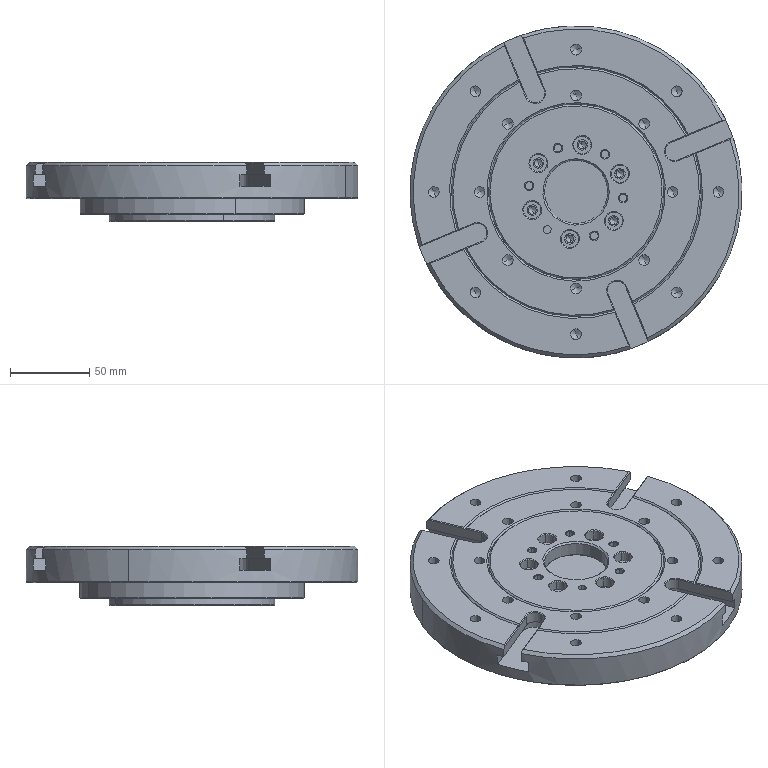NC program | Mastercam | posted with a generic post
Lines 3021 to 3620 of 4738:
(8 FEMF |TOOL - 9|DIA. OFF. - 9|LEN. - 9|TOOL DIA. - 8.)
N6098 T9 M6
N6100 G0 G54 G90 X17.184 Y2.469 C0. B0. S3500 M3
N6102 G43 H9 Z64.45
N6104 Z15.45
N6106 G1 Z14.45 F2000.
N6108 G41 D9 X14.616 Y-.598 F600.
N6110 G3 X14.594 Y-.645 I.077 J-.065
N6112 G1 X14.035 Y-3.838
N6114 X13.662 Y-4.467
N6116 G2 X.255 Y-12.103 I-13.407 J7.951
N6118 X-.045 Y-12.1 J15.587
N6120 X-12.1 Y0. I.045 J12.1
N6122 X-8.614 Y8.498 I12.1
N6124 G3 X-8.588 Y8.543 I-.071 J.07
N6126 G1 G40 X-7.579 Y12.413
N6128 G0 Z64.45
N6130 X17.184 Y2.469
N6132 Z15.45
N6134 G1 Z14.45 F2000.
N6136 G41 D9 X14.616 Y-.598 F600.
N6138 G3 X14.594 Y-.645 I.077 J-.065
N6140 G1 X14.035 Y-3.838
N6142 X13.662 Y-4.467
N6144 G2 X.255 Y-12.103 I-13.407 J7.951
N6146 X-.045 Y-12.1 J15.587
N6148 X-12.1 Y0. I.045 J12.1
N6150 X-8.614 Y8.498 I12.1
N6152 G3 X-8.588 Y8.543 I-.071 J.07
N6154 G1 G40 X-7.579 Y12.413
N6156 G0 Z64.45
N6158 C8.2 B-90.
N6160 X9.88 Y12.106
N6162 Z52.35
N6164 Z3.35
N6166 G1 Z2.35 F2000.
N6168 G41 D9 X9.521 Y8.122 F600.
N6170 G3 X9.5 Y7.657 I5.159 J-.465
N6172 X10.533 Y4.554 I5.18
N6174 G2 X12.001 Y.143 I-5.895 J-4.411
N6176 X10.828 Y-3.842 I-7.363
N6178 G3 X9.494 Y-8.378 I7.046 J-4.536
N6180 X9.5 Y-8.689 I8.38
N6182 G1 G40 X9.649 Y-12.687
N6184 G0 Z52.35
N6186 X9.88 Y12.106
N6188 Z3.35
N6190 G1 Z2.35 F2000.
N6192 G41 D9 X9.521 Y8.122 F600.
N6194 G3 X9.5 Y7.657 I5.159 J-.465
N6196 X10.533 Y4.554 I5.18
N6198 G2 X12.001 Y.143 I-5.895 J-4.411
N6200 X10.828 Y-3.842 I-7.363
N6202 G3 X9.494 Y-8.378 I7.046 J-4.536
N6204 X9.5 Y-8.689 I8.38
N6206 G1 G40 X9.649 Y-12.687
N6208 G0 Z52.35
N6210 X8.084 Y14.292
N6212 Z51.6
N6214 Z2.6
N6216 G1 Z-8.4 F2000.
N6218 G41 D9 X9.387 Y10.51 F600.
N6220 G3 X11.312 Y9.137 I1.925 J.663
N6222 X12.291 Y9.388 J2.036
N6224 G1 X18.686 Y13.541
N6226 G2 X21. Y14.226 I2.314 J-3.565
N6228 X25.25 Y9.976 J-4.25
N6230 X25.248 Y9.827 I-4.25
N6232 G1 Y9.82
N6234 G3 X25.44 Y9.62 I.199
N6236 G1 G40 X29.438 Y9.48
N6238 G0 Z41.6
N6240 X8.084 Y14.292
N6242 Z2.6
N6244 G1 Z-8.4 F2000.
N6246 G41 D9 X9.387 Y10.51 F600.
N6248 G3 X11.312 Y9.137 I1.925 J.663
N6250 X12.291 Y9.388 J2.036
N6252 G1 X18.686 Y13.541
N6254 G2 X21. Y14.226 I2.314 J-3.565
N6256 X25.25 Y9.976 J-4.25
N6258 X25.248 Y9.827 I-4.25
N6260 G1 Y9.82
N6262 G3 X25.44 Y9.62 I.199
N6264 G1 G40 X29.438 Y9.48
N6266 G0 Z51.6
N6268 Z57.06
N6270 X7.26 Y7.762
N6272 C0.
N6274 Z8.06
N6276 G1 Z7.06 F2000.
N6278 G41 D9 Y3.762 F600.
N6280 Y-3.762
N6282 G40 Y-7.762
N6284 G0 Z57.06
N6286 S3000 M3
N6288 C-.095 B-87.702
N6290 X25.467 Y13.177
N6292 Z42.615
N6294 Z-6.385
N6296 G1 Z-7.385 F2000.
N6298 G41 D9 X25.384 Y11.178 F400.
N6300 X24.716 Y-4.985
N6302 G40 X24.634 Y-6.983
N6304 G0 Z42.615
N6306 S3500 M3
N6308 Z50.
N6310 X3.874 Y8.762
N6312 C0. B-60.
N6314 Z11.234
N6316 G1 Z9.234 F2000.
N6318 G41 D9 Y3.762 F400.
N6320 Y-3.172
N6322 G40 Y-8.172
N6324 G0 Z50.
N6326 Z57.333
N6328 X-6.602 Y-7.762
N6330 B-45.
N6332 Z8.333
N6334 G1 Z7.333 F2000.
N6336 G41 D9 Y-3.762 F600.
N6338 Y3.762
N6340 G40 Y7.762
N6342 G0 Z57.333
N6344 Z58.
N6346 X-5.21 Y-14.199
N6348 B90.
N6350 Z9.
N6352 G1 Z-4. F2000.
N6354 G41 D9 X-7.914 Y-11.251 F600.
N6356 G3 X-14.089 Y-8.536 I-6.175 J-5.665
N6358 G1 X-16.963
N6360 G2 X-24.983 Y-.564 J8.02
N6362 G1 X-25.396 Y11.072
N6364 G3 X-25.398 Y11.089 I-.1 J-.004
N6366 G1 G40 X-26.232 Y15.001
N6368 G0 Z46.
N6370 X-5.21 Y-14.199
N6372 Z9.
N6374 G1 Z-4. F2000.
N6376 G41 D9 X-7.914 Y-11.251 F600.
N6378 G3 X-14.089 Y-8.536 I-6.175 J-5.665
N6380 G1 X-16.963
N6382 G2 X-24.983 Y-.564 J8.02
N6384 G1 X-25.396 Y11.072
N6386 G3 X-25.398 Y11.089 I-.1 J-.004
N6388 G1 G40 X-26.232 Y15.001
N6390 G0 Z58.
N6392 M5
N6394 G0 G28 G91 Z0.
N6396 G28 B0.
N6398 M01
N6400 G0 G17 G40 G80 G90 G94 G98
N6402 G0 G28 G91 Z0.
(12 R0.8 |TOOL - 10|DIA. OFF. - 10|LEN. - 10|TOOL DIA. - 12.)
N6404 T10 M6
N6406 G0 G54 G90 X17.851 Y-17.986 C8.2 B-90. S3500 M3
N6408 G43 H10 Z51.6
N6410 Z2.6
N6412 G1 Z1.6 F2000.
N6414 X17.494 Y-8.392 F400.
N6416 Y-8.378
N6418 G2 X17.555 Y-8.172 I.38
N6420 G3 X20. Y.143 I-12.917 J8.315
N6422 X17.537 Y8.486 I-15.362
N6424 G1 X12.374 Y17.504
N6426 X11.513 Y7.942
N6428 G3 X11.5 Y7.657 I3.167 J-.285
N6430 X12.134 Y5.752 I3.18
N6432 G2 X14. Y.143 I-7.496 J-5.609
N6434 X12.51 Y-4.924 I-9.362
N6436 G3 X11.494 Y-8.378 I5.364 J-3.454
N6438 X11.499 Y-8.615 I6.38
N6440 G1 X11.855 Y-18.208
N6442 G0 Z51.6
N6444 M5
N6446 G0 G28 G91 Z0.
N6448 G28 C0. B0.
N6450 M01
N6452 G0 G17 G40 G80 G90 G94 G98
N6454 G0 G28 G91 Z0.
(2 FEMF |TOOL - 7|DIA. OFF. - 7|LEN. - 7|TOOL DIA. - 2.)
N6456 T7 M6
N6458 G0 G54 G90 X22.009 Y12.644 C8.2 B-90. S5000 M3
N6460 G43 H7 Z50.
N6462 Z2.9
N6464 G1 Z-.73 F2000.
N6466 G41 D7 X21.744 Y12.22 F600.
N6468 X18.376 Y6.829
N6470 X18.32 Y5.236
N6472 X19.773 Y6.18
N6474 X23.215 Y11.688
N6476 G40 X23.48 Y12.112
N6478 X24.328 Y11.583
N6480 G42 D7 X24.063 Y11.159
N6482 X20.504 Y5.462
N6484 X17.254 Y3.352
N6486 X17.386 Y7.132
N6488 X20.896 Y12.75
N6490 G40 X21.161 Y13.174
N6492 X20.313 Y13.704
N6494 G41 D7 X20.048 Y13.28
N6496 X16.396 Y7.435
N6498 X16.215 Y2.25
N6500 X15.092 Y.228
N6502 G3 X15.043 Y.039 I.341 J-.189
N6504 X15.433 Y-.351 I.39
N6506 X15.774 Y-.15 J.39
N6508 G1 X16.945 Y1.959
N6510 X21.234 Y4.744
N6512 X24.911 Y10.629
N6514 G40 X25.176 Y11.053
N6516 G0 Z50.
N6518 X22.009 Y12.644
N6520 Z2.9
N6522 G1 Z-.78
N6524 G41 D7 X21.744 Y12.22
N6526 X18.376 Y6.829
N6528 X18.32 Y5.236
N6530 X19.773 Y6.18
N6532 X23.215 Y11.688
N6534 G40 X23.48 Y12.112
N6536 X24.328 Y11.583
N6538 G42 D7 X24.063 Y11.159
N6540 X20.504 Y5.462
N6542 X17.254 Y3.352
N6544 X17.386 Y7.132
N6546 X20.896 Y12.75
N6548 G40 X21.161 Y13.174
N6550 X20.313 Y13.704
N6552 G41 D7 X20.048 Y13.28
N6554 X16.396 Y7.435
N6556 X16.215 Y2.25
N6558 X15.092 Y.228
N6560 G3 X15.043 Y.039 I.341 J-.189
N6562 X15.433 Y-.351 I.39
N6564 X15.774 Y-.15 J.39
N6566 G1 X16.945 Y1.959
N6568 X21.234 Y4.744
N6570 X24.911 Y10.629
N6572 G40 X25.176 Y11.053
N6574 G0 Z50.
N6576 X22.009 Y12.644
N6578 Z2.9
N6580 G1 Z-.78
N6582 G41 D7 X21.744 Y12.22
N6584 X18.376 Y6.829
N6586 X18.32 Y5.236
N6588 X19.773 Y6.18
N6590 X23.215 Y11.688
N6592 G40 X23.48 Y12.112
N6594 X24.328 Y11.583
N6596 G42 D7 X24.063 Y11.159
N6598 X20.504 Y5.462
N6600 X17.254 Y3.352
N6602 X17.386 Y7.132
N6604 X20.896 Y12.75
N6606 G40 X21.161 Y13.174
N6608 X20.313 Y13.704
N6610 G41 D7 X20.048 Y13.28
N6612 X16.396 Y7.435
N6614 X16.215 Y2.25
N6616 X15.092 Y.228
N6618 G3 X15.043 Y.039 I.341 J-.189
N6620 X15.433 Y-.351 I.39
N6622 X15.774 Y-.15 J.39
N6624 G1 X16.945 Y1.959
N6626 X21.234 Y4.744
N6628 X24.911 Y10.629
N6630 G40 X25.176 Y11.053
N6632 G0 Z50.
N6634 M5
N6636 G0 G28 G91 Z0.
N6638 G28 C0. B0.
N6640 M01
N6642 G0 G17 G40 G80 G90 G94 G98
N6644 G0 G28 G91 Z0.
(6 XXXX |TOOL - 8|DIA. OFF. - 8|LEN. - 8|TOOL DIA. - 6.)
N6646 T8 M6
N6648 G0 G54 G90 X16.632 Y9.573 C8.2 B-90. S3000 M3
N6650 G43 H8 Z50.034
N6652 Z1.034
N6654 G1 Z-.466 F2000.
N6656 G41 D8 X16.527 Y6.575 F400.
N6658 X16.36 Y1.771
N6660 X20.425 Y4.411
N6662 G40 X22.941 Y6.045
N6664 X16.532 Y9.577
N6666 G41 D8 X16.427 Y6.579
N6668 X16.253 Y1.582
N6670 X20.48 Y4.327
N6672 G40 X22.996 Y5.961
N6674 G0 Z50.034
N6676 M5
N6678 G0 G28 G91 Z0.
N6680 G28 C0. B0.
N6682 M01
N6684 G0 G17 G40 G80 G90 G94 G98
N6686 G0 G28 G91 Z0.
(5 CHM |TOOL - 12|DIA. OFF. - 12|LEN. - 12|TOOL DIA. - 5.)
N6688 T12 M6
N6690 G0 G54 G90 X18.253 Y5.128 C8.2 B-90. S2000 M3
N6692 G43 H12 Z29.22
N6694 G81 G98 Z-2.28 R.22 F100.
N6696 G80
N6698 M5
N6700 G0 G28 G91 Z0.
N6702 G28 C0. B0.
N6704 M01
N6706 G0 G17 G40 G80 G90 G94 G98
N6708 G0 G28 G91 Z0.
(2.1 DR |TOOL - 13|DIA. OFF. - 13|LEN. - 13|TOOL DIA. - 2.1)
N6710 T13 M6
N6712 G0 G54 G90 X18.253 Y5.128 C8.2 B-90. S2500 M3
N6714 G43 H13 Z29.22
N6716 G83 G98 Z-8.28 R.22 Q1. F60.
N6718 G80
N6720 M5
N6722 G0 G28 G91 Z0.
N6724 G28 C0. B0.
N6726 M01
N6728 G0 G17 G40 G80 G90 G94 G98
N6730 G0 G28 G91 Z0.
(3 FEM |TOOL - 11|DIA. OFF. - 11|LEN. - 11|TOOL DIA. - 3.)
N6732 T11 M6
N6734 G0 G54 G90 X18.253 Y-5.128 C188.2 B-90. S2000 M3
N6736 G43 H11 Z37.278
N6738 G81 G98 Z5.278 R8.278 F100.
N6740 G80
N6742 M5
N6744 G0 G28 G91 Z0.
N6746 G28 C0. B0.
N6748 M01
N6750 G0 G17 G40 G80 G90 G94 G98
N6752 G0 G28 G91 Z0.
(1.95 THML |TOOL - 14|DIA. OFF. - 14|LEN. - 14|TOOL DIA. - 1.95)
N6754 T14 M6
N6756 G0 G54 G90 X18.253 Y5.128 C8.2 B-90. S3000 M3
N6758 G43 H14 Z29.22
N6760 Z1.22
N6762 G1 Z-6.28 F2000.
N6764 G41 D14 X18.403 F40.
N6766 G3 X18.253 Y5.278 Z-6.168 I-.15
N6768 X18.103 Y5.128 Z-6.055 J-.15
N6770 X18.253 Y4.978 Z-5.942 I.15
N6772 X18.403 Y5.128 Z-5.83 J.15
N6774 X18.253 Y5.278 Z-5.718 I-.15
N6776 X18.103 Y5.128 Z-5.605 J-.15
N6778 G1 G40 X18.253
N6780 Z-4.93 F2000.
N6782 G41 D14 X18.403 F40.
N6784 G3 X18.253 Y5.278 Z-4.817 I-.15
N6786 X18.103 Y5.128 Z-4.705 J-.15
N6788 X18.253 Y4.978 Z-4.593 I.15
N6790 X18.403 Y5.128 Z-4.48 J.15
N6792 X18.253 Y5.278 Z-4.367 I-.15
N6794 X18.103 Y5.128 Z-4.255 J-.15
N6796 G1 G40 X18.253
N6798 Z-3.58 F2000.
N6800 G41 D14 X18.403 F40.
N6802 G3 X18.253 Y5.278 Z-3.467 I-.15
N6804 X18.103 Y5.128 Z-3.355 J-.15
N6806 X18.253 Y4.978 Z-3.243 I.15
N6808 X18.403 Y5.128 Z-3.131 J.15
N6810 X18.253 Y5.278 Z-3.018 I-.15
N6812 X18.103 Y5.128 Z-2.905 J-.15
N6814 G1 G40 X18.253
N6816 Z-2.23 F2000.
N6818 G41 D14 X18.403 F40.
N6820 G3 X18.253 Y5.278 Z-2.118 I-.15
N6822 X18.103 Y5.128 Z-2.005 J-.15
N6824 X18.253 Y4.978 Z-1.893 I.15
N6826 X18.403 Y5.128 Z-1.78 J.15
N6828 X18.253 Y5.278 Z-1.667 I-.15
N6830 X18.103 Y5.128 Z-1.555 J-.15
N6832 G1 G40 X18.253
N6834 Z-6.28 F2000.
N6836 G41 D14 X18.428 F40.
N6838 G3 X18.253 Y5.303 Z-6.168 I-.175
N6840 X18.078 Y5.128 Z-6.055 J-.175
N6842 X18.253 Y4.953 Z-5.942 I.175
N6844 X18.428 Y5.128 Z-5.83 J.175
N6846 X18.253 Y5.303 Z-5.718 I-.175
N6848 X18.078 Y5.128 Z-5.605 J-.175
N6850 G1 G40 X18.253
N6852 Z-4.93 F2000.
N6854 G41 D14 X18.428 F40.
N6856 G3 X18.253 Y5.303 Z-4.817 I-.175
N6858 X18.078 Y5.128 Z-4.705 J-.175
N6860 X18.253 Y4.953 Z-4.593 I.175
N6862 X18.428 Y5.128 Z-4.48 J.175
N6864 X18.253 Y5.303 Z-4.367 I-.175
N6866 X18.078 Y5.128 Z-4.255 J-.175
N6868 G1 G40 X18.253
N6870 Z-3.58 F2000.
N6872 G41 D14 X18.428 F40.
N6874 G3 X18.253 Y5.303 Z-3.467 I-.175
N6876 X18.078 Y5.128 Z-3.355 J-.175
N6878 X18.253 Y4.953 Z-3.243 I.175
N6880 X18.428 Y5.128 Z-3.131 J.175
N6882 X18.253 Y5.303 Z-3.018 I-.175
N6884 X18.078 Y5.128 Z-2.905 J-.175
N6886 G1 G40 X18.253
N6888 Z-2.23 F2000.
N6890 G41 D14 X18.428 F40.
N6892 G3 X18.253 Y5.303 Z-2.118 I-.175
N6894 X18.078 Y5.128 Z-2.005 J-.175
N6896 X18.253 Y4.953 Z-1.893 I.175
N6898 X18.428 Y5.128 Z-1.78 J.175
N6900 X18.253 Y5.303 Z-1.667 I-.175
N6902 X18.078 Y5.128 Z-1.555 J-.175
N6904 G1 G40 X18.253
N6906 Z-6.28 F2000.
N6908 G41 D14 X18.453 F40.
N6910 G3 X18.253 Y5.328 Z-6.168 I-.2
N6912 X18.053 Y5.128 Z-6.055 J-.2
N6914 X18.253 Y4.928 Z-5.942 I.2
N6916 X18.453 Y5.128 Z-5.83 J.2
N6918 X18.253 Y5.328 Z-5.718 I-.2
N6920 X18.053 Y5.128 Z-5.605 J-.2
N6922 G1 G40 X18.253
N6924 Z-4.93 F2000.
N6926 G41 D14 X18.453 F40.
N6928 G3 X18.253 Y5.328 Z-4.817 I-.2
N6930 X18.053 Y5.128 Z-4.705 J-.2
N6932 X18.253 Y4.928 Z-4.593 I.2
N6934 X18.453 Y5.128 Z-4.48 J.2
N6936 X18.253 Y5.328 Z-4.367 I-.2
N6938 X18.053 Y5.128 Z-4.255 J-.2
N6940 G1 G40 X18.253
N6942 Z-3.58 F2000.
N6944 G41 D14 X18.453 F40.
N6946 G3 X18.253 Y5.328 Z-3.467 I-.2
N6948 X18.053 Y5.128 Z-3.355 J-.2
N6950 X18.253 Y4.928 Z-3.243 I.2
N6952 X18.453 Y5.128 Z-3.131 J.2
N6954 X18.253 Y5.328 Z-3.018 I-.2
N6956 X18.053 Y5.128 Z-2.905 J-.2
N6958 G1 G40 X18.253
N6960 Z-2.23 F2000.
N6962 G41 D14 X18.453 F40.
N6964 G3 X18.253 Y5.328 Z-2.118 I-.2
N6966 X18.053 Y5.128 Z-2.005 J-.2
N6968 X18.253 Y4.928 Z-1.893 I.2
N6970 X18.453 Y5.128 Z-1.78 J.2
N6972 X18.253 Y5.328 Z-1.667 I-.2
N6974 X18.053 Y5.128 Z-1.555 J-.2
N6976 G1 G40 X18.253
N6978 Z-6.28 F2000.
N6980 G41 D14 X18.478 F40.
N6982 G3 X18.253 Y5.353 Z-6.168 I-.225
N6984 X18.028 Y5.128 Z-6.055 J-.225
N6986 X18.253 Y4.903 Z-5.942 I.225
N6988 X18.478 Y5.128 Z-5.83 J.225
N6990 X18.253 Y5.353 Z-5.718 I-.225
N6992 X18.028 Y5.128 Z-5.605 J-.225
N6994 G1 G40 X18.253
N6996 Z-4.93 F2000.
N6998 G41 D14 X18.478 F40.
N7000 G3 X18.253 Y5.353 Z-4.817 I-.225
N7002 X18.028 Y5.128 Z-4.705 J-.225
N7004 X18.253 Y4.903 Z-4.593 I.225
N7006 X18.478 Y5.128 Z-4.48 J.225
N7008 X18.253 Y5.353 Z-4.367 I-.225
N7010 X18.028 Y5.128 Z-4.255 J-.225
N7012 G1 G40 X18.253
N7014 Z-3.58 F2000.
N7016 G41 D14 X18.478 F40.
N7018 G3 X18.253 Y5.353 Z-3.467 I-.225
N7020 X18.028 Y5.128 Z-3.355 J-.225
N7022 X18.253 Y4.903 Z-3.243 I.225
N7024 X18.478 Y5.128 Z-3.131 J.225
N7026 X18.253 Y5.353 Z-3.018 I-.225
N7028 X18.028 Y5.128 Z-2.905 J-.225
N7030 G1 G40 X18.253
N7032 Z-2.23 F2000.
N7034 G41 D14 X18.478 F40.
N7036 G3 X18.253 Y5.353 Z-2.118 I-.225
N7038 X18.028 Y5.128 Z-2.005 J-.225
N7040 X18.253 Y4.903 Z-1.893 I.225
N7042 X18.478 Y5.128 Z-1.78 J.225
N7044 X18.253 Y5.353 Z-1.667 I-.225
N7046 X18.028 Y5.128 Z-1.555 J-.225
N7048 G1 G40 X18.253
N7050 Z-6.28 F2000.
N7052 G41 D14 X18.503 F40.
N7054 G3 X18.253 Y5.378 Z-6.168 I-.25
N7056 X18.003 Y5.128 Z-6.055 J-.25
N7058 X18.253 Y4.878 Z-5.942 I.25
N7060 X18.503 Y5.128 Z-5.83 J.25
N7062 X18.253 Y5.378 Z-5.718 I-.25
N7064 X18.003 Y5.128 Z-5.605 J-.25
N7066 G1 G40 X18.253
N7068 Z-4.93 F2000.
N7070 G41 D14 X18.503 F40.
N7072 G3 X18.253 Y5.378 Z-4.817 I-.25
N7074 X18.003 Y5.128 Z-4.705 J-.25
N7076 X18.253 Y4.878 Z-4.593 I.25
N7078 X18.503 Y5.128 Z-4.48 J.25
N7080 X18.253 Y5.378 Z-4.367 I-.25
N7082 X18.003 Y5.128 Z-4.255 J-.25
N7084 G1 G40 X18.253
N7086 Z-3.58 F2000.
N7088 G41 D14 X18.503 F40.
N7090 G3 X18.253 Y5.378 Z-3.467 I-.25
N7092 X18.003 Y5.128 Z-3.355 J-.25
N7094 X18.253 Y4.878 Z-3.243 I.25
N7096 X18.503 Y5.128 Z-3.131 J.25
N7098 X18.253 Y5.378 Z-3.018 I-.25
N7100 X18.003 Y5.128 Z-2.905 J-.25
N7102 G1 G40 X18.253
N7104 Z-2.23 F2000.
N7106 G41 D14 X18.503 F40.
N7108 G3 X18.253 Y5.378 Z-2.118 I-.25
N7110 X18.003 Y5.128 Z-2.005 J-.25
N7112 X18.253 Y4.878 Z-1.893 I.25
N7114 X18.503 Y5.128 Z-1.78 J.25
N7116 X18.253 Y5.378 Z-1.667 I-.25
N7118 X18.003 Y5.128 Z-1.555 J-.25
N7120 G1 G40 X18.253
N7122 Z-6.28 F2000.
N7124 G41 D14 X18.528 F40.
N7126 G3 X18.253 Y5.403 Z-6.168 I-.275
N7128 X17.978 Y5.128 Z-6.055 J-.275
N7130 X18.253 Y4.853 Z-5.942 I.275
N7132 X18.528 Y5.128 Z-5.83 J.275
N7134 X18.253 Y5.403 Z-5.718 I-.275
N7136 X17.978 Y5.128 Z-5.605 J-.275
N7138 G1 G40 X18.253
N7140 Z-4.93 F2000.
N7142 G41 D14 X18.528 F40.
N7144 G3 X18.253 Y5.403 Z-4.817 I-.275
N7146 X17.978 Y5.128 Z-4.705 J-.275
N7148 X18.253 Y4.853 Z-4.593 I.275
N7150 X18.528 Y5.128 Z-4.48 J.275
N7152 X18.253 Y5.403 Z-4.367 I-.275
N7154 X17.978 Y5.128 Z-4.255 J-.275
N7156 G1 G40 X18.253
N7158 Z-3.58 F2000.
N7160 G41 D14 X18.528 F40.
N7162 G3 X18.253 Y5.403 Z-3.467 I-.275
N7164 X17.978 Y5.128 Z-3.355 J-.275
N7166 X18.253 Y4.853 Z-3.243 I.275
N7168 X18.528 Y5.128 Z-3.131 J.275
N7170 X18.253 Y5.403 Z-3.018 I-.275
N7172 X17.978 Y5.128 Z-2.905 J-.275
N7174 G1 G40 X18.253
N7176 Z-2.23 F2000.
N7178 G41 D14 X18.528 F40.
N7180 G3 X18.253 Y5.403 Z-2.118 I-.275
N7182 X17.978 Y5.128 Z-2.005 J-.275
N7184 X18.253 Y4.853 Z-1.893 I.275
N7186 X18.528 Y5.128 Z-1.78 J.275
N7188 X18.253 Y5.403 Z-1.667 I-.275
N7190 X17.978 Y5.128 Z-1.555 J-.275
N7192 G1 G40 X18.253
N7194 Z-6.28 F2000.
N7196 G41 D14 X18.528 F40.
N7198 G3 X18.253 Y5.403 Z-6.168 I-.275
N7200 X17.978 Y5.128 Z-6.055 J-.275
N7202 X18.253 Y4.853 Z-5.942 I.275
N7204 X18.528 Y5.128 Z-5.83 J.275
N7206 X18.253 Y5.403 Z-5.718 I-.275
N7208 X17.978 Y5.128 Z-5.605 J-.275
N7210 G1 G40 X18.253
N7212 Z-4.93 F2000.
N7214 G41 D14 X18.528 F40.
N7216 G3 X18.253 Y5.403 Z-4.817 I-.275
N7218 X17.978 Y5.128 Z-4.705 J-.275
N7220 X18.253 Y4.853 Z-4.593 I.275
N7222 X18.528 Y5.128 Z-4.48 J.275
N7224 X18.253 Y5.403 Z-4.367 I-.275
N7226 X17.978 Y5.128 Z-4.255 J-.275
N7228 G1 G40 X18.253
N7230 Z-3.58 F2000.
N7232 G41 D14 X18.528 F40.
N7234 G3 X18.253 Y5.403 Z-3.467 I-.275
N7236 X17.978 Y5.128 Z-3.355 J-.275
N7238 X18.253 Y4.853 Z-3.243 I.275
N7240 X18.528 Y5.128 Z-3.131 J.275
N7242 X18.253 Y5.403 Z-3.018 I-.275
N7244 X17.978 Y5.128 Z-2.905 J-.275
N7246 G1 G40 X18.253
N7248 Z-2.23 F2000.
N7250 G41 D14 X18.528 F40.
N7252 G3 X18.253 Y5.403 Z-2.118 I-.275
N7254 X17.978 Y5.128 Z-2.005 J-.275
N7256 X18.253 Y4.853 Z-1.893 I.275
N7258 X18.528 Y5.128 Z-1.78 J.275
N7260 X18.253 Y5.403 Z-1.667 I-.275
N7262 X17.978 Y5.128 Z-1.555 J-.275
N7264 G1 G40 X18.253
N7266 G0 Z1.22
N7268 Z29.22
N7270 M5
N7272 G0 G28 G91 Z0.
N7274 G28 C0. B0.
N7276 M01
N7278 G0 G17 G40 G80 G90 G94 G98
N7280 G0 G28 G91 Z0.